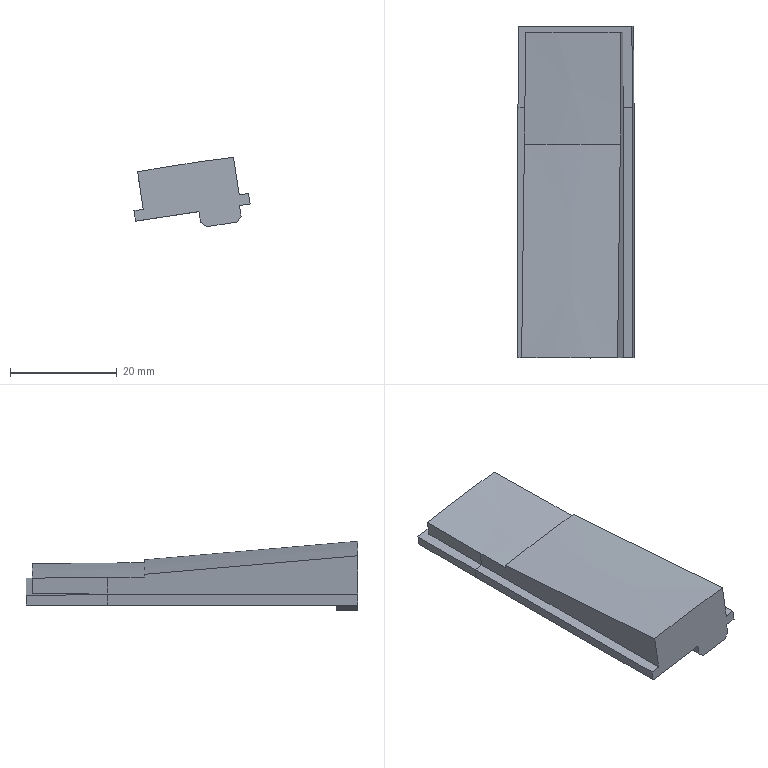Part | STEP file | 1 solid | 24 faces | box 21.719 x 62.11 x 12.971 mm | volume 7839 mm3 | plane 22 | cone 2